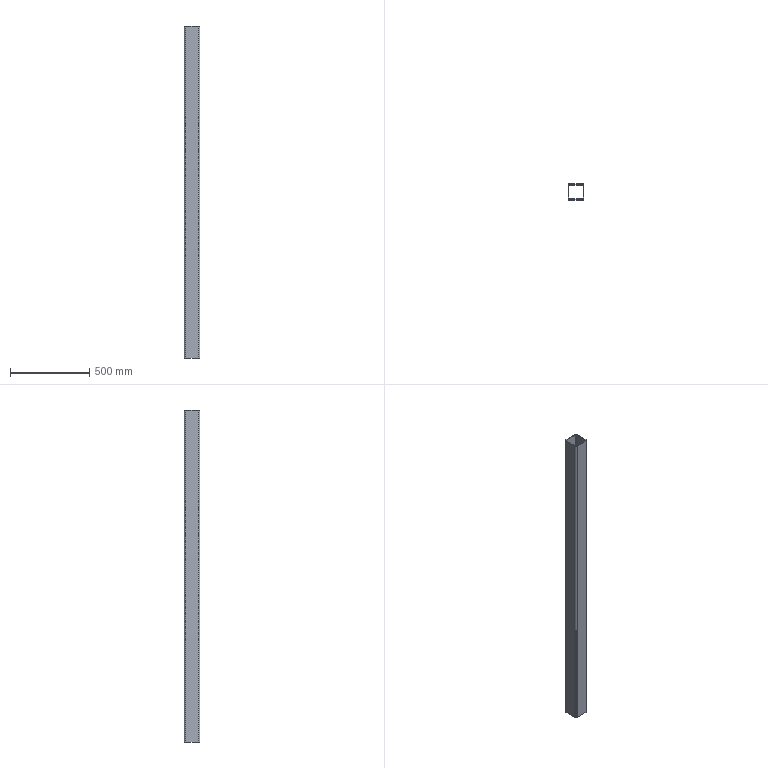Part | SolidWorks | features Extrusion 1 | 1 solid | 18 faces | box 100 x 100 x 2100 mm | volume 3854801 mm3 | plane 10 | cylinder 8 | commonest cylinder face diameters 10 x4 20 x4
STEP:
#1=CARTESIAN_POINT('',(-40.,50.,1050.));
#2=VERTEX_POINT('',#1);
#3=CARTESIAN_POINT('',(-50.,40.,1050.));
#4=VERTEX_POINT('',#3);
#5=CARTESIAN_POINT('',(-40.,40.,1050.));
#6=DIRECTION('',(0.,0.,1.));
#7=DIRECTION('',(1.,0.,0.));
#8=AXIS2_PLACEMENT_3D('',#5,#6,#7);
#9=CIRCLE('',#8,10.);
#10=EDGE_CURVE('',#2,#4,#9,.T.);
#11=ORIENTED_EDGE('',*,*,#10,.T.);
#12=CARTESIAN_POINT('',(-50.,-40.,1050.));
#13=VERTEX_POINT('',#12);
#14=CARTESIAN_POINT('',(-50.,40.,1050.));
#15=DIRECTION('',(0.,-1.,0.));
#16=VECTOR('',#15,1000.);
#17=LINE('',#14,#16);
#18=EDGE_CURVE('',#4,#13,#17,.T.);
#19=ORIENTED_EDGE('',*,*,#18,.T.);
#20=CARTESIAN_POINT('',(-40.,-50.,1050.));
#21=VERTEX_POINT('',#20);
#22=CARTESIAN_POINT('',(-40.,-40.,1050.));
#23=DIRECTION('',(0.,0.,1.));
#24=DIRECTION('',(-1.,0.,0.));
#25=AXIS2_PLACEMENT_3D('',#22,#23,#24);
#26=CIRCLE('',#25,10.);
#27=EDGE_CURVE('',#13,#21,#26,.T.);
#28=ORIENTED_EDGE('',*,*,#27,.T.);
#29=CARTESIAN_POINT('',(40.,-50.,1050.));
#30=VERTEX_POINT('',#29);
#31=CARTESIAN_POINT('',(40.,-50.,1050.));
#32=DIRECTION('',(1.,0.,0.));
#33=VECTOR('',#32,1000.);
#34=LINE('',#31,#33);
#35=EDGE_CURVE('',#21,#30,#34,.T.);
#36=ORIENTED_EDGE('',*,*,#35,.T.);
#37=CARTESIAN_POINT('',(50.,-40.,1050.));
#38=VERTEX_POINT('',#37);
#39=CARTESIAN_POINT('',(40.,-40.,1050.));
#40=DIRECTION('',(0.,0.,1.));
#41=DIRECTION('',(1.,0.,0.));
#42=AXIS2_PLACEMENT_3D('',#39,#40,#41);
#43=CIRCLE('',#42,10.);
#44=EDGE_CURVE('',#30,#38,#43,.T.);
#45=ORIENTED_EDGE('',*,*,#44,.T.);
#46=CARTESIAN_POINT('',(50.,40.,1050.));
#47=VERTEX_POINT('',#46);
#48=CARTESIAN_POINT('',(50.,-40.,1050.));
#49=DIRECTION('',(0.,1.,0.));
#50=VECTOR('',#49,1000.);
#51=LINE('',#48,#50);
#52=EDGE_CURVE('',#38,#47,#51,.T.);
#53=ORIENTED_EDGE('',*,*,#52,.T.);
#54=CARTESIAN_POINT('',(40.,50.,1050.));
#55=VERTEX_POINT('',#54);
#56=CARTESIAN_POINT('',(40.,40.,1050.));
#57=DIRECTION('',(0.,0.,1.));
#58=DIRECTION('',(-1.,0.,0.));
#59=AXIS2_PLACEMENT_3D('',#56,#57,#58);
#60=CIRCLE('',#59,10.);
#61=EDGE_CURVE('',#47,#55,#60,.T.);
#62=ORIENTED_EDGE('',*,*,#61,.T.);
#63=CARTESIAN_POINT('',(0.,50.,1050.));
#64=DIRECTION('',(-1.,0.,0.));
#65=VECTOR('',#64,1000.);
#66=LINE('',#63,#65);
#67=EDGE_CURVE('',#55,#2,#66,.T.);
#68=ORIENTED_EDGE('',*,*,#67,.T.);
#69=EDGE_LOOP('',(#11,#19,#28,#36,#45,#53,#62,#68));
#70=FACE_OUTER_BOUND('',#69,.T.);
#71=CARTESIAN_POINT('',(-45.,40.,1050.));
#72=VERTEX_POINT('',#71);
#73=CARTESIAN_POINT('',(-45.,-40.,1050.));
#74=VERTEX_POINT('',#73);
#75=CARTESIAN_POINT('',(-45.,40.,1050.));
#76=DIRECTION('',(0.,-1.,0.));
#77=VECTOR('',#76,1000.);
#78=LINE('',#75,#77);
#79=EDGE_CURVE('',#72,#74,#78,.T.);
#80=ORIENTED_EDGE('',*,*,#79,.F.);
#81=CARTESIAN_POINT('',(-40.,45.,1050.));
#82=VERTEX_POINT('',#81);
#83=CARTESIAN_POINT('',(-40.,40.,1050.));
#84=DIRECTION('',(0.,0.,1.));
#85=DIRECTION('',(1.,0.,0.));
#86=AXIS2_PLACEMENT_3D('',#83,#84,#85);
#87=CIRCLE('',#86,5.);
#88=EDGE_CURVE('',#82,#72,#87,.T.);
#89=ORIENTED_EDGE('',*,*,#88,.F.);
#90=CARTESIAN_POINT('',(40.,45.,1050.));
#91=VERTEX_POINT('',#90);
#92=CARTESIAN_POINT('',(0.,45.,1050.));
#93=DIRECTION('',(-1.,0.,0.));
#94=VECTOR('',#93,1000.);
#95=LINE('',#92,#94);
#96=EDGE_CURVE('',#91,#82,#95,.T.);
#97=ORIENTED_EDGE('',*,*,#96,.F.);
#98=CARTESIAN_POINT('',(45.,40.,1050.));
#99=VERTEX_POINT('',#98);
#100=CARTESIAN_POINT('',(40.,40.,1050.));
#101=DIRECTION('',(0.,0.,1.));
#102=DIRECTION('',(-1.,0.,0.));
#103=AXIS2_PLACEMENT_3D('',#100,#101,#102);
#104=CIRCLE('',#103,5.);
#105=EDGE_CURVE('',#99,#91,#104,.T.);
#106=ORIENTED_EDGE('',*,*,#105,.F.);
#107=CARTESIAN_POINT('',(45.,-40.,1050.));
#108=VERTEX_POINT('',#107);
#109=CARTESIAN_POINT('',(45.,-40.,1050.));
#110=DIRECTION('',(0.,1.,0.));
#111=VECTOR('',#110,1000.);
#112=LINE('',#109,#111);
#113=EDGE_CURVE('',#108,#99,#112,.T.);
#114=ORIENTED_EDGE('',*,*,#113,.F.);
#115=CARTESIAN_POINT('',(40.,-45.,1050.));
#116=VERTEX_POINT('',#115);
#117=CARTESIAN_POINT('',(40.,-40.,1050.));
#118=DIRECTION('',(0.,0.,1.));
#119=DIRECTION('',(1.,0.,0.));
#120=AXIS2_PLACEMENT_3D('',#117,#118,#119);
#121=CIRCLE('',#120,5.);
#122=EDGE_CURVE('',#116,#108,#121,.T.);
#123=ORIENTED_EDGE('',*,*,#122,.F.);
#124=CARTESIAN_POINT('',(-40.,-45.,1050.));
#125=VERTEX_POINT('',#124);
#126=CARTESIAN_POINT('',(40.,-45.,1050.));
#127=DIRECTION('',(1.,0.,0.));
#128=VECTOR('',#127,1000.);
#129=LINE('',#126,#128);
#130=EDGE_CURVE('',#125,#116,#129,.T.);
#131=ORIENTED_EDGE('',*,*,#130,.F.);
#132=CARTESIAN_POINT('',(-40.,-40.,1050.));
#133=DIRECTION('',(0.,0.,1.));
#134=DIRECTION('',(-1.,0.,0.));
#135=AXIS2_PLACEMENT_3D('',#132,#133,#134);
#136=CIRCLE('',#135,5.);
#137=EDGE_CURVE('',#74,#125,#136,.T.);
#138=ORIENTED_EDGE('',*,*,#137,.F.);
#139=EDGE_LOOP('',(#80,#89,#97,#106,#114,#123,#131,#138));
#140=FACE_BOUND('',#139,.T.);
#141=CARTESIAN_POINT('',(-40.,40.,1050.));
#142=DIRECTION('',(0.,0.,1.));
#143=DIRECTION('',(1.,0.,0.));
#144=AXIS2_PLACEMENT_3D('',#141,#142,#143);
#145=PLANE('',#144);
#146=ADVANCED_FACE('',(#70,#140),#145,.T.);
#147=CARTESIAN_POINT('',(-40.,50.,-1050.));
#148=VERTEX_POINT('',#147);
#149=CARTESIAN_POINT('',(-50.,40.,-1050.));
#150=VERTEX_POINT('',#149);
#151=CARTESIAN_POINT('',(-40.,40.,-1050.));
#152=DIRECTION('',(0.,0.,1.));
#153=DIRECTION('',(1.,0.,0.));
#154=AXIS2_PLACEMENT_3D('',#151,#152,#153);
#155=CIRCLE('',#154,10.);
#156=EDGE_CURVE('',#148,#150,#155,.T.);
#157=ORIENTED_EDGE('',*,*,#156,.F.);
#158=CARTESIAN_POINT('',(40.,50.,-1050.));
#159=VERTEX_POINT('',#158);
#160=CARTESIAN_POINT('',(0.,50.,-1050.));
#161=DIRECTION('',(-1.,0.,0.));
#162=VECTOR('',#161,1000.);
#163=LINE('',#160,#162);
#164=EDGE_CURVE('',#159,#148,#163,.T.);
#165=ORIENTED_EDGE('',*,*,#164,.F.);
#166=CARTESIAN_POINT('',(50.,40.,-1050.));
#167=VERTEX_POINT('',#166);
#168=CARTESIAN_POINT('',(40.,40.,-1050.));
#169=DIRECTION('',(0.,0.,1.));
#170=DIRECTION('',(-1.,0.,0.));
#171=AXIS2_PLACEMENT_3D('',#168,#169,#170);
#172=CIRCLE('',#171,10.);
#173=EDGE_CURVE('',#167,#159,#172,.T.);
#174=ORIENTED_EDGE('',*,*,#173,.F.);
#175=CARTESIAN_POINT('',(50.,-40.,-1050.));
#176=VERTEX_POINT('',#175);
#177=CARTESIAN_POINT('',(50.,40.,-1050.));
#178=DIRECTION('',(0.,1.,0.));
#179=VECTOR('',#178,1000.);
#180=LINE('',#177,#179);
#181=EDGE_CURVE('',#176,#167,#180,.T.);
#182=ORIENTED_EDGE('',*,*,#181,.F.);
#183=CARTESIAN_POINT('',(40.,-50.,-1050.));
#184=VERTEX_POINT('',#183);
#185=CARTESIAN_POINT('',(40.,-40.,-1050.));
#186=DIRECTION('',(0.,0.,1.));
#187=DIRECTION('',(1.,0.,0.));
#188=AXIS2_PLACEMENT_3D('',#185,#186,#187);
#189=CIRCLE('',#188,10.);
#190=EDGE_CURVE('',#184,#176,#189,.T.);
#191=ORIENTED_EDGE('',*,*,#190,.F.);
#192=CARTESIAN_POINT('',(-40.,-50.,-1050.));
#193=VERTEX_POINT('',#192);
#194=CARTESIAN_POINT('',(40.,-50.,-1050.));
#195=DIRECTION('',(1.,0.,0.));
#196=VECTOR('',#195,1000.);
#197=LINE('',#194,#196);
#198=EDGE_CURVE('',#193,#184,#197,.T.);
#199=ORIENTED_EDGE('',*,*,#198,.F.);
#200=CARTESIAN_POINT('',(-50.,-40.,-1050.));
#201=VERTEX_POINT('',#200);
#202=CARTESIAN_POINT('',(-40.,-40.,-1050.));
#203=DIRECTION('',(0.,0.,1.));
#204=DIRECTION('',(-1.,0.,0.));
#205=AXIS2_PLACEMENT_3D('',#202,#203,#204);
#206=CIRCLE('',#205,10.);
#207=EDGE_CURVE('',#201,#193,#206,.T.);
#208=ORIENTED_EDGE('',*,*,#207,.F.);
#209=CARTESIAN_POINT('',(-50.,-40.,-1050.));
#210=DIRECTION('',(0.,-1.,0.));
#211=VECTOR('',#210,1000.);
#212=LINE('',#209,#211);
#213=EDGE_CURVE('',#150,#201,#212,.T.);
#214=ORIENTED_EDGE('',*,*,#213,.F.);
#215=EDGE_LOOP('',(#157,#165,#174,#182,#191,#199,#208,#214));
#216=FACE_OUTER_BOUND('',#215,.T.);
#217=CARTESIAN_POINT('',(-40.,45.,-1050.));
#218=VERTEX_POINT('',#217);
#219=CARTESIAN_POINT('',(-45.,40.,-1050.));
#220=VERTEX_POINT('',#219);
#221=CARTESIAN_POINT('',(-40.,40.,-1050.));
#222=DIRECTION('',(0.,0.,1.));
#223=DIRECTION('',(1.,0.,0.));
#224=AXIS2_PLACEMENT_3D('',#221,#222,#223);
#225=CIRCLE('',#224,5.);
#226=EDGE_CURVE('',#218,#220,#225,.T.);
#227=ORIENTED_EDGE('',*,*,#226,.T.);
#228=CARTESIAN_POINT('',(-45.,-40.,-1050.));
#229=VERTEX_POINT('',#228);
#230=CARTESIAN_POINT('',(-45.,-40.,-1050.));
#231=DIRECTION('',(0.,-1.,0.));
#232=VECTOR('',#231,1000.);
#233=LINE('',#230,#232);
#234=EDGE_CURVE('',#220,#229,#233,.T.);
#235=ORIENTED_EDGE('',*,*,#234,.T.);
#236=CARTESIAN_POINT('',(-40.,-45.,-1050.));
#237=VERTEX_POINT('',#236);
#238=CARTESIAN_POINT('',(-40.,-40.,-1050.));
#239=DIRECTION('',(0.,0.,1.));
#240=DIRECTION('',(-1.,0.,0.));
#241=AXIS2_PLACEMENT_3D('',#238,#239,#240);
#242=CIRCLE('',#241,5.);
#243=EDGE_CURVE('',#229,#237,#242,.T.);
#244=ORIENTED_EDGE('',*,*,#243,.T.);
#245=CARTESIAN_POINT('',(40.,-45.,-1050.));
#246=VERTEX_POINT('',#245);
#247=CARTESIAN_POINT('',(40.,-45.,-1050.));
#248=DIRECTION('',(1.,0.,0.));
#249=VECTOR('',#248,1000.);
#250=LINE('',#247,#249);
#251=EDGE_CURVE('',#237,#246,#250,.T.);
#252=ORIENTED_EDGE('',*,*,#251,.T.);
#253=CARTESIAN_POINT('',(45.,-40.,-1050.));
#254=VERTEX_POINT('',#253);
#255=CARTESIAN_POINT('',(40.,-40.,-1050.));
#256=DIRECTION('',(0.,0.,1.));
#257=DIRECTION('',(1.,0.,0.));
#258=AXIS2_PLACEMENT_3D('',#255,#256,#257);
#259=CIRCLE('',#258,5.);
#260=EDGE_CURVE('',#246,#254,#259,.T.);
#261=ORIENTED_EDGE('',*,*,#260,.T.);
#262=CARTESIAN_POINT('',(45.,40.,-1050.));
#263=VERTEX_POINT('',#262);
#264=CARTESIAN_POINT('',(45.,40.,-1050.));
#265=DIRECTION('',(0.,1.,0.));
#266=VECTOR('',#265,1000.);
#267=LINE('',#264,#266);
#268=EDGE_CURVE('',#254,#263,#267,.T.);
#269=ORIENTED_EDGE('',*,*,#268,.T.);
#270=CARTESIAN_POINT('',(40.,45.,-1050.));
#271=VERTEX_POINT('',#270);
#272=CARTESIAN_POINT('',(40.,40.,-1050.));
#273=DIRECTION('',(0.,0.,1.));
#274=DIRECTION('',(-1.,0.,0.));
#275=AXIS2_PLACEMENT_3D('',#272,#273,#274);
#276=CIRCLE('',#275,5.);
#277=EDGE_CURVE('',#263,#271,#276,.T.);
#278=ORIENTED_EDGE('',*,*,#277,.T.);
#279=CARTESIAN_POINT('',(0.,45.,-1050.));
#280=DIRECTION('',(-1.,0.,0.));
#281=VECTOR('',#280,1000.);
#282=LINE('',#279,#281);
#283=EDGE_CURVE('',#271,#218,#282,.T.);
#284=ORIENTED_EDGE('',*,*,#283,.T.);
#285=EDGE_LOOP('',(#227,#235,#244,#252,#261,#269,#278,#284));
#286=FACE_BOUND('',#285,.T.);
#287=CARTESIAN_POINT('',(-40.,40.,-1050.));
#288=DIRECTION('',(0.,0.,1.));
#289=DIRECTION('',(1.,0.,0.));
#290=AXIS2_PLACEMENT_3D('',#287,#288,#289);
#291=PLANE('',#290);
#292=ADVANCED_FACE('',(#216,#286),#291,.F.);
#293=ORIENTED_EDGE('',*,*,#156,.T.);
#294=CARTESIAN_POINT('',(-50.,40.,1050.));
#295=DIRECTION('',(0.,0.,-1.));
#296=VECTOR('',#295,1000.);
#297=LINE('',#294,#296);
#298=EDGE_CURVE('',#4,#150,#297,.T.);
#299=ORIENTED_EDGE('',*,*,#298,.F.);
#300=ORIENTED_EDGE('',*,*,#10,.F.);
#301=CARTESIAN_POINT('',(-40.,50.,1050.));
#302=DIRECTION('',(0.,0.,-1.));
#303=VECTOR('',#302,1000.);
#304=LINE('',#301,#303);
#305=EDGE_CURVE('',#2,#148,#304,.T.);
#306=ORIENTED_EDGE('',*,*,#305,.T.);
#307=EDGE_LOOP('',(#293,#299,#300,#306));
#308=FACE_OUTER_BOUND('',#307,.T.);
#309=CARTESIAN_POINT('',(-40.,40.,1050.));
#310=DIRECTION('',(0.,0.,-1.));
#311=DIRECTION('',(-1.,0.,0.));
#312=AXIS2_PLACEMENT_3D('',#309,#310,#311);
#313=CYLINDRICAL_SURFACE('',#312,10.);
#314=ADVANCED_FACE('',(#308),#313,.T.);
#315=ORIENTED_EDGE('',*,*,#213,.T.);
#316=CARTESIAN_POINT('',(-50.,-40.,1050.));
#317=DIRECTION('',(0.,0.,-1.));
#318=VECTOR('',#317,1000.);
#319=LINE('',#316,#318);
#320=EDGE_CURVE('',#13,#201,#319,.T.);
#321=ORIENTED_EDGE('',*,*,#320,.F.);
#322=ORIENTED_EDGE('',*,*,#18,.F.);
#323=ORIENTED_EDGE('',*,*,#298,.T.);
#324=EDGE_LOOP('',(#315,#321,#322,#323));
#325=FACE_OUTER_BOUND('',#324,.T.);
#326=CARTESIAN_POINT('',(-50.,-40.,1050.));
#327=DIRECTION('',(1.,0.,0.));
#328=DIRECTION('',(0.,1.,0.));
#329=AXIS2_PLACEMENT_3D('',#326,#327,#328);
#330=PLANE('',#329);
#331=ADVANCED_FACE('',(#325),#330,.F.);
#332=ORIENTED_EDGE('',*,*,#207,.T.);
#333=CARTESIAN_POINT('',(-40.,-50.,1050.));
#334=DIRECTION('',(0.,0.,-1.));
#335=VECTOR('',#334,1000.);
#336=LINE('',#333,#335);
#337=EDGE_CURVE('',#21,#193,#336,.T.);
#338=ORIENTED_EDGE('',*,*,#337,.F.);
#339=ORIENTED_EDGE('',*,*,#27,.F.);
#340=ORIENTED_EDGE('',*,*,#320,.T.);
#341=EDGE_LOOP('',(#332,#338,#339,#340));
#342=FACE_OUTER_BOUND('',#341,.T.);
#343=CARTESIAN_POINT('',(-40.,-40.,1050.));
#344=DIRECTION('',(0.,0.,-1.));
#345=DIRECTION('',(-1.,0.,0.));
#346=AXIS2_PLACEMENT_3D('',#343,#344,#345);
#347=CYLINDRICAL_SURFACE('',#346,10.);
#348=ADVANCED_FACE('',(#342),#347,.T.);
#349=ORIENTED_EDGE('',*,*,#198,.T.);
#350=CARTESIAN_POINT('',(40.,-50.,1050.));
#351=DIRECTION('',(0.,0.,-1.));
#352=VECTOR('',#351,1000.);
#353=LINE('',#350,#352);
#354=EDGE_CURVE('',#30,#184,#353,.T.);
#355=ORIENTED_EDGE('',*,*,#354,.F.);
#356=ORIENTED_EDGE('',*,*,#35,.F.);
#357=ORIENTED_EDGE('',*,*,#337,.T.);
#358=EDGE_LOOP('',(#349,#355,#356,#357));
#359=FACE_OUTER_BOUND('',#358,.T.);
#360=CARTESIAN_POINT('',(40.,-50.,1050.));
#361=DIRECTION('',(0.,1.,0.));
#362=DIRECTION('',(-1.,0.,0.));
#363=AXIS2_PLACEMENT_3D('',#360,#361,#362);
#364=PLANE('',#363);
#365=ADVANCED_FACE('',(#359),#364,.F.);
#366=ORIENTED_EDGE('',*,*,#190,.T.);
#367=CARTESIAN_POINT('',(50.,-40.,1050.));
#368=DIRECTION('',(0.,0.,-1.));
#369=VECTOR('',#368,1000.);
#370=LINE('',#367,#369);
#371=EDGE_CURVE('',#38,#176,#370,.T.);
#372=ORIENTED_EDGE('',*,*,#371,.F.);
#373=ORIENTED_EDGE('',*,*,#44,.F.);
#374=ORIENTED_EDGE('',*,*,#354,.T.);
#375=EDGE_LOOP('',(#366,#372,#373,#374));
#376=FACE_OUTER_BOUND('',#375,.T.);
#377=CARTESIAN_POINT('',(40.,-40.,1050.));
#378=DIRECTION('',(0.,0.,-1.));
#379=DIRECTION('',(-1.,0.,0.));
#380=AXIS2_PLACEMENT_3D('',#377,#378,#379);
#381=CYLINDRICAL_SURFACE('',#380,10.);
#382=ADVANCED_FACE('',(#376),#381,.T.);
#383=ORIENTED_EDGE('',*,*,#181,.T.);
#384=CARTESIAN_POINT('',(50.,40.,1050.));
#385=DIRECTION('',(0.,0.,-1.));
#386=VECTOR('',#385,1000.);
#387=LINE('',#384,#386);
#388=EDGE_CURVE('',#47,#167,#387,.T.);
#389=ORIENTED_EDGE('',*,*,#388,.F.);
#390=ORIENTED_EDGE('',*,*,#52,.F.);
#391=ORIENTED_EDGE('',*,*,#371,.T.);
#392=EDGE_LOOP('',(#383,#389,#390,#391));
#393=FACE_OUTER_BOUND('',#392,.T.);
#394=CARTESIAN_POINT('',(50.,40.,1050.));
#395=DIRECTION('',(-1.,0.,0.));
#396=DIRECTION('',(0.,-1.,0.));
#397=AXIS2_PLACEMENT_3D('',#394,#395,#396);
#398=PLANE('',#397);
#399=ADVANCED_FACE('',(#393),#398,.F.);
#400=ORIENTED_EDGE('',*,*,#173,.T.);
#401=CARTESIAN_POINT('',(40.,50.,1050.));
#402=DIRECTION('',(0.,0.,-1.));
#403=VECTOR('',#402,1000.);
#404=LINE('',#401,#403);
#405=EDGE_CURVE('',#55,#159,#404,.T.);
#406=ORIENTED_EDGE('',*,*,#405,.F.);
#407=ORIENTED_EDGE('',*,*,#61,.F.);
#408=ORIENTED_EDGE('',*,*,#388,.T.);
#409=EDGE_LOOP('',(#400,#406,#407,#408));
#410=FACE_OUTER_BOUND('',#409,.T.);
#411=CARTESIAN_POINT('',(40.,40.,1050.));
#412=DIRECTION('',(0.,0.,-1.));
#413=DIRECTION('',(-1.,0.,0.));
#414=AXIS2_PLACEMENT_3D('',#411,#412,#413);
#415=CYLINDRICAL_SURFACE('',#414,10.);
#416=ADVANCED_FACE('',(#410),#415,.T.);
#417=ORIENTED_EDGE('',*,*,#164,.T.);
#418=ORIENTED_EDGE('',*,*,#305,.F.);
#419=ORIENTED_EDGE('',*,*,#67,.F.);
#420=ORIENTED_EDGE('',*,*,#405,.T.);
#421=EDGE_LOOP('',(#417,#418,#419,#420));
#422=FACE_OUTER_BOUND('',#421,.T.);
#423=CARTESIAN_POINT('',(0.,50.,1050.));
#424=DIRECTION('',(0.,-1.,0.));
#425=DIRECTION('',(1.,0.,0.));
#426=AXIS2_PLACEMENT_3D('',#423,#424,#425);
#427=PLANE('',#426);
#428=ADVANCED_FACE('',(#422),#427,.F.);
#429=ORIENTED_EDGE('',*,*,#226,.F.);
#430=CARTESIAN_POINT('',(-40.,45.,1050.));
#431=DIRECTION('',(0.,0.,-1.));
#432=VECTOR('',#431,1000.);
#433=LINE('',#430,#432);
#434=EDGE_CURVE('',#82,#218,#433,.T.);
#435=ORIENTED_EDGE('',*,*,#434,.F.);
#436=ORIENTED_EDGE('',*,*,#88,.T.);
#437=CARTESIAN_POINT('',(-45.,40.,1050.));
#438=DIRECTION('',(0.,0.,-1.));
#439=VECTOR('',#438,1000.);
#440=LINE('',#437,#439);
#441=EDGE_CURVE('',#72,#220,#440,.T.);
#442=ORIENTED_EDGE('',*,*,#441,.T.);
#443=EDGE_LOOP('',(#429,#435,#436,#442));
#444=FACE_OUTER_BOUND('',#443,.T.);
#445=CARTESIAN_POINT('',(-40.,40.,1050.));
#446=DIRECTION('',(0.,0.,-1.));
#447=DIRECTION('',(-1.,0.,0.));
#448=AXIS2_PLACEMENT_3D('',#445,#446,#447);
#449=CYLINDRICAL_SURFACE('',#448,5.);
#450=ADVANCED_FACE('',(#444),#449,.F.);
#451=ORIENTED_EDGE('',*,*,#234,.F.);
#452=ORIENTED_EDGE('',*,*,#441,.F.);
#453=ORIENTED_EDGE('',*,*,#79,.T.);
#454=CARTESIAN_POINT('',(-45.,-40.,1050.));
#455=DIRECTION('',(0.,0.,-1.));
#456=VECTOR('',#455,1000.);
#457=LINE('',#454,#456);
#458=EDGE_CURVE('',#74,#229,#457,.T.);
#459=ORIENTED_EDGE('',*,*,#458,.T.);
#460=EDGE_LOOP('',(#451,#452,#453,#459));
#461=FACE_OUTER_BOUND('',#460,.T.);
#462=CARTESIAN_POINT('',(-45.,-40.,1050.));
#463=DIRECTION('',(1.,0.,0.));
#464=DIRECTION('',(0.,0.,-1.));
#465=AXIS2_PLACEMENT_3D('',#462,#463,#464);
#466=PLANE('',#465);
#467=ADVANCED_FACE('',(#461),#466,.T.);
#468=ORIENTED_EDGE('',*,*,#243,.F.);
#469=ORIENTED_EDGE('',*,*,#458,.F.);
#470=ORIENTED_EDGE('',*,*,#137,.T.);
#471=CARTESIAN_POINT('',(-40.,-45.,1050.));
#472=DIRECTION('',(0.,0.,-1.));
#473=VECTOR('',#472,1000.);
#474=LINE('',#471,#473);
#475=EDGE_CURVE('',#125,#237,#474,.T.);
#476=ORIENTED_EDGE('',*,*,#475,.T.);
#477=EDGE_LOOP('',(#468,#469,#470,#476));
#478=FACE_OUTER_BOUND('',#477,.T.);
#479=CARTESIAN_POINT('',(-40.,-40.,1050.));
#480=DIRECTION('',(0.,0.,-1.));
#481=DIRECTION('',(-1.,0.,0.));
#482=AXIS2_PLACEMENT_3D('',#479,#480,#481);
#483=CYLINDRICAL_SURFACE('',#482,5.);
#484=ADVANCED_FACE('',(#478),#483,.F.);
#485=ORIENTED_EDGE('',*,*,#251,.F.);
#486=ORIENTED_EDGE('',*,*,#475,.F.);
#487=ORIENTED_EDGE('',*,*,#130,.T.);
#488=CARTESIAN_POINT('',(40.,-45.,1050.));
#489=DIRECTION('',(0.,0.,-1.));
#490=VECTOR('',#489,1000.);
#491=LINE('',#488,#490);
#492=EDGE_CURVE('',#116,#246,#491,.T.);
#493=ORIENTED_EDGE('',*,*,#492,.T.);
#494=EDGE_LOOP('',(#485,#486,#487,#493));
#495=FACE_OUTER_BOUND('',#494,.T.);
#496=CARTESIAN_POINT('',(40.,-45.,1050.));
#497=DIRECTION('',(0.,1.,0.));
#498=DIRECTION('',(-1.,0.,0.));
#499=AXIS2_PLACEMENT_3D('',#496,#497,#498);
#500=PLANE('',#499);
#501=ADVANCED_FACE('',(#495),#500,.T.);
#502=ORIENTED_EDGE('',*,*,#260,.F.);
#503=ORIENTED_EDGE('',*,*,#492,.F.);
#504=ORIENTED_EDGE('',*,*,#122,.T.);
#505=CARTESIAN_POINT('',(45.,-40.,1050.));
#506=DIRECTION('',(0.,0.,-1.));
#507=VECTOR('',#506,1000.);
#508=LINE('',#505,#507);
#509=EDGE_CURVE('',#108,#254,#508,.T.);
#510=ORIENTED_EDGE('',*,*,#509,.T.);
#511=EDGE_LOOP('',(#502,#503,#504,#510));
#512=FACE_OUTER_BOUND('',#511,.T.);
#513=CARTESIAN_POINT('',(40.,-40.,1050.));
#514=DIRECTION('',(0.,0.,-1.));
#515=DIRECTION('',(-1.,0.,0.));
#516=AXIS2_PLACEMENT_3D('',#513,#514,#515);
#517=CYLINDRICAL_SURFACE('',#516,5.);
#518=ADVANCED_FACE('',(#512),#517,.F.);
#519=ORIENTED_EDGE('',*,*,#268,.F.);
#520=ORIENTED_EDGE('',*,*,#509,.F.);
#521=ORIENTED_EDGE('',*,*,#113,.T.);
#522=CARTESIAN_POINT('',(45.,40.,1050.));
#523=DIRECTION('',(0.,0.,-1.));
#524=VECTOR('',#523,1000.);
#525=LINE('',#522,#524);
#526=EDGE_CURVE('',#99,#263,#525,.T.);
#527=ORIENTED_EDGE('',*,*,#526,.T.);
#528=EDGE_LOOP('',(#519,#520,#521,#527));
#529=FACE_OUTER_BOUND('',#528,.T.);
#530=CARTESIAN_POINT('',(45.,40.,1050.));
#531=DIRECTION('',(-1.,0.,0.));
#532=DIRECTION('',(0.,0.,1.));
#533=AXIS2_PLACEMENT_3D('',#530,#531,#532);
#534=PLANE('',#533);
#535=ADVANCED_FACE('',(#529),#534,.T.);
#536=ORIENTED_EDGE('',*,*,#277,.F.);
#537=ORIENTED_EDGE('',*,*,#526,.F.);
#538=ORIENTED_EDGE('',*,*,#105,.T.);
#539=CARTESIAN_POINT('',(40.,45.,1050.));
#540=DIRECTION('',(0.,0.,-1.));
#541=VECTOR('',#540,1000.);
#542=LINE('',#539,#541);
#543=EDGE_CURVE('',#91,#271,#542,.T.);
#544=ORIENTED_EDGE('',*,*,#543,.T.);
#545=EDGE_LOOP('',(#536,#537,#538,#544));
#546=FACE_OUTER_BOUND('',#545,.T.);
#547=CARTESIAN_POINT('',(40.,40.,1050.));
#548=DIRECTION('',(0.,0.,-1.));
#549=DIRECTION('',(-1.,0.,0.));
#550=AXIS2_PLACEMENT_3D('',#547,#548,#549);
#551=CYLINDRICAL_SURFACE('',#550,5.);
#552=ADVANCED_FACE('',(#546),#551,.F.);
#553=ORIENTED_EDGE('',*,*,#283,.F.);
#554=ORIENTED_EDGE('',*,*,#543,.F.);
#555=ORIENTED_EDGE('',*,*,#96,.T.);
#556=ORIENTED_EDGE('',*,*,#434,.T.);
#557=EDGE_LOOP('',(#553,#554,#555,#556));
#558=FACE_OUTER_BOUND('',#557,.T.);
#559=CARTESIAN_POINT('',(0.,45.,1050.));
#560=DIRECTION('',(0.,-1.,0.));
#561=DIRECTION('',(1.,0.,0.));
#562=AXIS2_PLACEMENT_3D('',#559,#560,#561);
#563=PLANE('',#562);
#564=ADVANCED_FACE('',(#558),#563,.T.);
#565=CLOSED_SHELL('',(#146,#292,#314,#331,#348,#365,#382,#399,#416,#428,#450,#467,#484,#501,#518,#535,#552,#564));
#566=MANIFOLD_SOLID_BREP('',#565);
#567=CARTESIAN_POINT('',(0.,0.,0.));
#568=DIRECTION('',(0.,0.,1.));
#569=DIRECTION('',(1.,0.,0.));
#570=AXIS2_PLACEMENT_3D('',#567,#568,#569);
#571=(LENGTH_UNIT()NAMED_UNIT(*)SI_UNIT(.MILLI.,.METRE.));
#572=UNCERTAINTY_MEASURE_WITH_UNIT(LENGTH_MEASURE(0.00001),#571,'','');
#573=(NAMED_UNIT(*)PLANE_ANGLE_UNIT()SI_UNIT($,.RADIAN.));
#574=(NAMED_UNIT(*)SI_UNIT($,.STERADIAN.)SOLID_ANGLE_UNIT());
#575=(GEOMETRIC_REPRESENTATION_CONTEXT(3)GLOBAL_UNCERTAINTY_ASSIGNED_CONTEXT((#572))GLOBAL_UNIT_ASSIGNED_CONTEXT((#571,#573,#574))REPRESENTATION_CONTEXT('',''));
#576=ADVANCED_BREP_SHAPE_REPRESENTATION('',(#566,#570),#575);